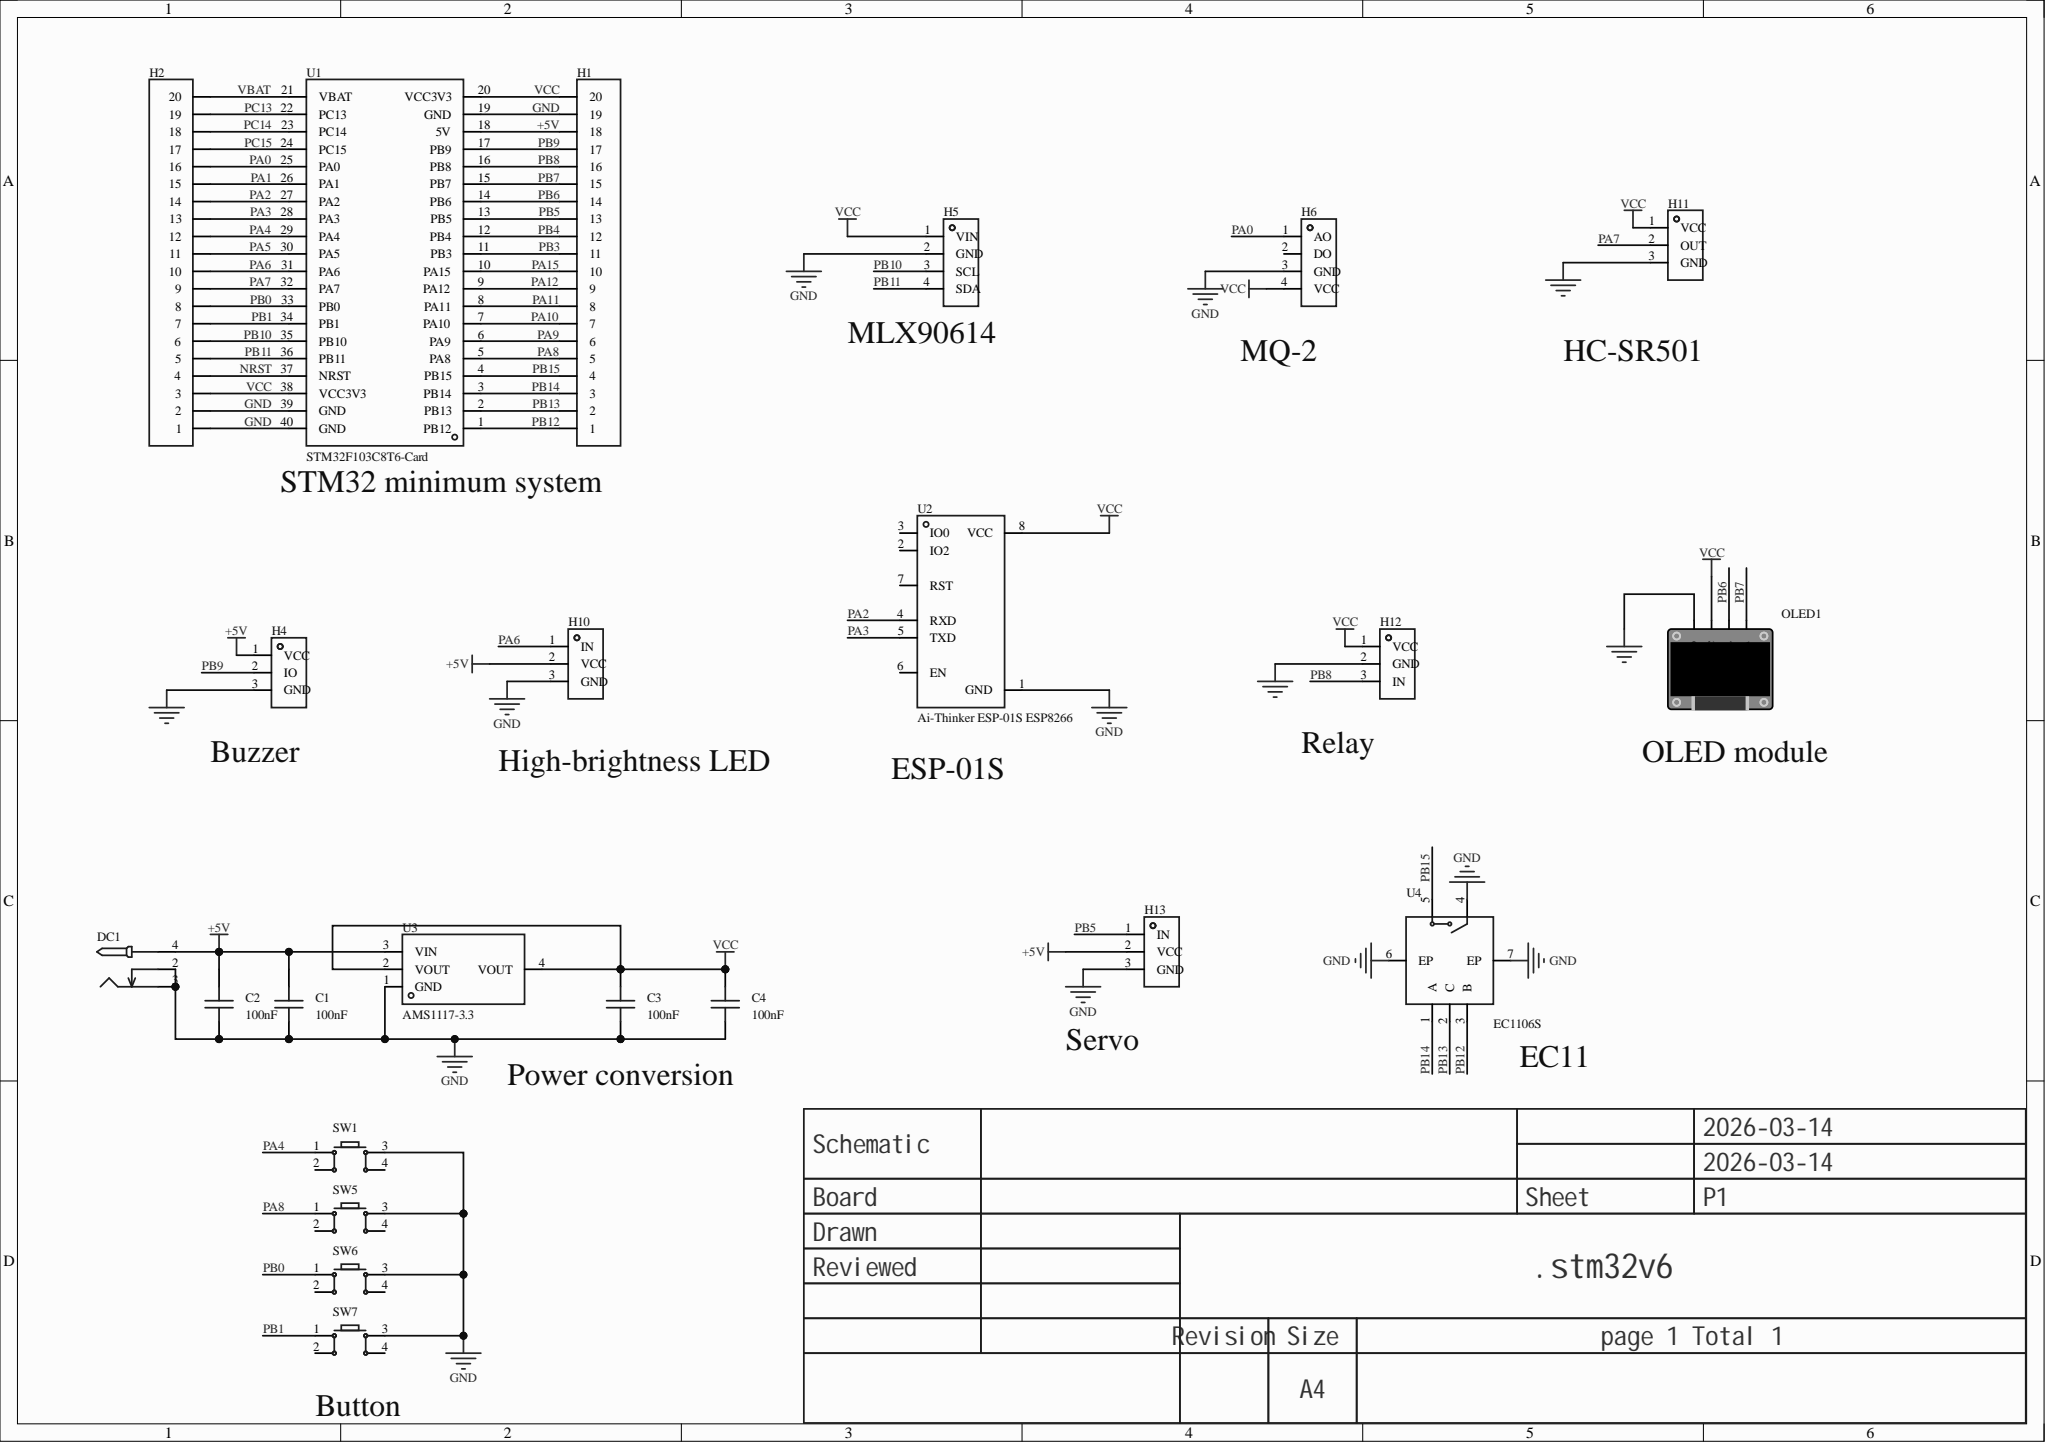Circuit board | Altium Designer | 23 parts | 37 nets
Bill of materials:
Comment,Description,Designator,Footprint,LibRef,Quantity
"100nF","","C1, C2, C3, C4","C0603","CAP_0603","4"
"","","DC1","DC-2.0","DC-005_2.0","1"
"","","H1, H2","HDR-TH_20P-P2.54-V-F","HDR-F_2.54_1x20P","2"
"","","H4, H10, H11, H12, H13","HDR-TH_3P-P2.54-V-F","HDR-F_2.54_1x3P","5"
"","","H5, H6","HDR-TH_4P-P2.54-V-F","HDR-F_2.54_1x4P","2"
"","","OLED1","0.96OLED_4P","0.96OLED模块_4P","1"
"","","SW1, SW5, SW6, SW7","SW-TH_4P-L6.0-W6.0-P4.50-LS6.5","Key_TH_6x6x6","4"
"STM32F103C8T6-Card","","U1","CONN-TH_L53.3-W22.9_STM32F103C8T6-CARD","STM32F103C8T6-Card","1"
"Ai-Thinker ESP-01S ESP8266","","U2","WIFIM-TH_8P-L24.7-W14.4-P2.54","Ai-Thinker ESP-01S ESP8266","1"
"AMS1117-3.3","Output type:Fixed;Operating voltage:-;Output voltage:3.3V;Output current:1A;Power supply rejection ratio (PSRR):72dB@(120Hz);Output polarity:Positive;","U3","SOT-223-3_L6.5-W3.4-P2.30-LS7.0-BR","AMS1117-3.3_C6186","1"
"EC1106S","","U4","SW-SMD_EC1106S","EC1106S","1"
Netlist (Protel format):
[
C1
C0603
100nF



]
[
C2
C0603
100nF



]
[
C3
C0603
100nF



]
[
C4
C0603
100nF



]
[
DC1
DC-2.0




]
[
H1
HDR-TH_20P-P2.54-V-F




]
[
H2
HDR-TH_20P-P2.54-V-F




]
[
H4
HDR-TH_3P-P2.54-V-F




]
[
H5
HDR-TH_4P-P2.54-V-F




]
[
H6
HDR-TH_4P-P2.54-V-F




]
[
H10
HDR-TH_3P-P2.54-V-F




]
[
H11
HDR-TH_3P-P2.54-V-F




]
[
H12
HDR-TH_3P-P2.54-V-F




]
[
H13
HDR-TH_3P-P2.54-V-F




]
[
OLED1
0.96OLED_4P




]
[
SW1
SW-TH_4P-L6.0-W6.0-P4.50-LS6.5




]
[
SW5
SW-TH_4P-L6.0-W6.0-P4.50-LS6.5




]
[
SW6
SW-TH_4P-L6.0-W6.0-P4.50-LS6.5




]
[
SW7
SW-TH_4P-L6.0-W6.0-P4.50-LS6.5




]
[
U1
CONN-TH_L53.3-W22.9_STM32F103C8T6-CARD
STM32F103C8T6-Card



]
[
U2
WIFIM-TH_8P-L24.7-W14.4-P2.54
Ai-Thinker ESP-01S ESP8266



]
[
U3
SOT-223-3_L6.5-W3.4-P2.30-LS7.0-BR
AMS1117-3.3



]
[
U4
SW-SMD_EC1106S
EC1106S



]
(
VCC
C3-2
C4-2
H1-20
H2-3
H5-1
H6-4
H11-1
H12-1
OLED1-2
U1-20
U1-38
U2-8
U3-2
U3-4
)
(
VBAT
H2-20
U1-21
)
(
PC15
H2-17
U1-24
)
(
PC14
H2-18
U1-23
)
(
PC13
H2-19
U1-22
)
(
PB15
H1-4
U1-4
U4-5
)
(
PB14
H1-3
U1-3
U4-1
)
(
PB13
H1-2
U1-2
U4-2
)
(
PB12
H1-1
U1-1
U4-3
)
(
PB11
H2-5
H5-4
U1-36
)
(
PB10
H2-6
H5-3
U1-35
)
(
PB9
H1-17
H4-2
U1-17
)
(
PB8
H1-16
H12-3
U1-16
)
(
PB7
H1-15
OLED1-4
U1-15
)
(
PB6
H1-14
OLED1-3
U1-14
)
(
PB5
H1-13
H13-1
U1-13
)
(
PB4
H1-12
U1-12
)
(
PB3
H1-11
U1-11
)
(
PB1
H2-7
SW7-1
U1-34
)
(
PB0
H2-8
SW6-1
U1-33
)
(
PA15
H1-10
U1-10
)
(
PA12
H1-9
U1-9
)
(
PA11
H1-8
U1-8
)
(
PA10
H1-7
U1-7
)
(
PA9
H1-6
U1-6
)
(
PA8
H1-5
SW5-1
U1-5
)
(
PA7
H2-9
H11-2
U1-32
)
(
PA6
H2-10
H10-1
U1-31
)
(
PA5
H2-11
U1-30
)
(
PA4
H2-12
SW1-1
U1-29
)
(
PA3
H2-13
U1-28
U2-5
)
(
PA2
H2-14
U1-27
U2-4
)
(
PA1
H2-15
U1-26
)
(
PA0
H2-16
H6-1
U1-25
)
(
NRST
H2-4
U1-37
)
(
GND
C1-1
C2-1
C3-1
C4-1
DC1-2
DC1-3
H1-19
H2-1
H2-2
H4-3
H5-2
H6-3
H10-3
H11-3
H12-2
H13-3
OLED1-1
SW1-3
SW5-3
SW6-3
SW7-3
U1-19
U1-39
U1-40
U2-1
U3-1
U4-4
U4-6
U4-7
)
(
+5V
C1-2
C2-2
DC1-4
H1-18
H4-1
H10-2
H13-2
U1-18
U3-3
)